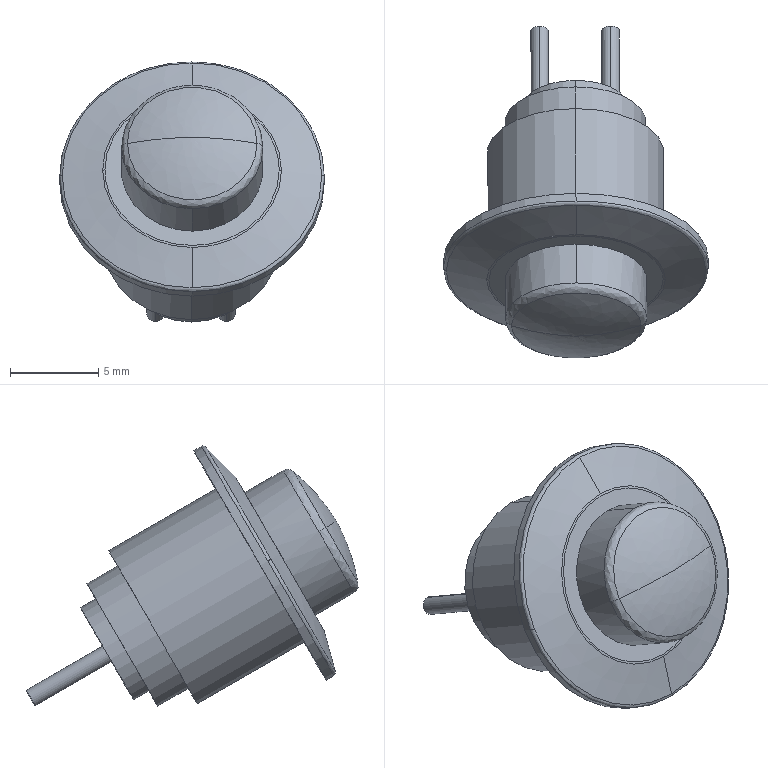Part | SolidWorks | features BaseBody 1 | 1 solid | 31 faces | box 15.002 x 18.816 x 14.734 mm | volume 1046 mm3 | cylinder 14 | spline 8 | plane 7 | cone 2 | commonest cylinder face diameters 1 x4 8 x4 6.02 x2 10 x2 15 x2
STEP:
#1=CARTESIAN_POINT('',(757.571,31.906,30.606));
#2=VERTEX_POINT('',#1);
#3=CARTESIAN_POINT('',(764.921,28.263,24.241));
#4=VERTEX_POINT('',#3);
#5=CARTESIAN_POINT('',(757.571,28.231,24.241));
#6=DIRECTION('',(-0.003769,0.866,-0.5));
#7=DIRECTION('',(-1.,-0.004352,0.000000001));
#8=AXIS2_PLACEMENT_3D('',#5,#6,#7);
#9=CIRCLE('',#8,7.35);
#10=EDGE_CURVE('',#2,#4,#9,.T.);
#11=ORIENTED_EDGE('',*,*,#10,.T.);
#12=CARTESIAN_POINT('',(765.07,28.431,24.144));
#13=VERTEX_POINT('',#12);
#14=CARTESIAN_POINT('',(764.87,28.43,24.144));
#15=DIRECTION('',(-0.002176,0.5,0.866));
#16=DIRECTION('',(1.,0.004352,-0.000000001));
#17=AXIS2_PLACEMENT_3D('',#14,#15,#16);
#18=CIRCLE('',#17,0.2);
#19=EDGE_CURVE('',#4,#13,#18,.T.);
#20=ORIENTED_EDGE('',*,*,#19,.T.);
#21=CARTESIAN_POINT('',(757.57,32.149,30.639));
#22=VERTEX_POINT('',#21);
#23=CARTESIAN_POINT('',(757.57,28.399,24.144));
#24=DIRECTION('',(-0.003769,0.866,-0.5));
#25=DIRECTION('',(0.,-0.5,-0.866));
#26=AXIS2_PLACEMENT_3D('',#23,#24,#25);
#27=CIRCLE('',#26,7.5);
#28=EDGE_CURVE('',#22,#13,#27,.T.);
#29=ORIENTED_EDGE('',*,*,#28,.F.);
#30=CARTESIAN_POINT('',(750.07,28.366,24.144));
#31=VERTEX_POINT('',#30);
#32=CARTESIAN_POINT('',(757.57,28.399,24.144));
#33=DIRECTION('',(-0.003769,0.866,-0.5));
#34=DIRECTION('',(0.,-0.5,-0.866));
#35=AXIS2_PLACEMENT_3D('',#32,#33,#34);
#36=CIRCLE('',#35,7.5);
#37=EDGE_CURVE('',#31,#22,#36,.T.);
#38=ORIENTED_EDGE('',*,*,#37,.F.);
#39=CARTESIAN_POINT('',(750.221,28.199,24.241));
#40=VERTEX_POINT('',#39);
#41=CARTESIAN_POINT('',(750.27,28.367,24.144));
#42=DIRECTION('',(0.002176,-0.5,-0.866));
#43=DIRECTION('',(-1.,-0.004352,0.000000001));
#44=AXIS2_PLACEMENT_3D('',#41,#42,#43);
#45=CIRCLE('',#44,0.2);
#46=EDGE_CURVE('',#40,#31,#45,.T.);
#47=ORIENTED_EDGE('',*,*,#46,.F.);
#48=CARTESIAN_POINT('',(757.571,28.231,24.241));
#49=DIRECTION('',(-0.003769,0.866,-0.5));
#50=DIRECTION('',(-1.,-0.004352,0.000000001));
#51=AXIS2_PLACEMENT_3D('',#48,#49,#50);
#52=CIRCLE('',#51,7.35);
#53=EDGE_CURVE('',#40,#2,#52,.T.);
#54=ORIENTED_EDGE('',*,*,#53,.T.);
#55=EDGE_LOOP('',(#11,#20,#29,#38,#47,#54));
#56=FACE_OUTER_BOUND('',#55,.T.);
#57=CARTESIAN_POINT('',(764.921,28.263,24.241));
#58=CARTESIAN_POINT('',(764.889,35.613,36.972));
#59=CARTESIAN_POINT('',(750.189,35.549,36.972));
#60=CARTESIAN_POINT('',(750.221,28.199,24.241));
#61=CARTESIAN_POINT('',(765.013,28.284,24.229));
#62=CARTESIAN_POINT('',(764.981,35.726,37.119));
#63=CARTESIAN_POINT('',(750.097,35.661,37.119));
#64=CARTESIAN_POINT('',(750.129,28.219,24.229));
#65=CARTESIAN_POINT('',(765.071,28.349,24.191));
#66=CARTESIAN_POINT('',(765.038,35.849,37.182));
#67=CARTESIAN_POINT('',(750.038,35.784,37.182));
#68=CARTESIAN_POINT('',(750.071,28.284,24.191));
#69=CARTESIAN_POINT('',(765.07,28.431,24.144));
#70=CARTESIAN_POINT('',(765.038,35.931,37.134));
#71=CARTESIAN_POINT('',(750.038,35.866,37.134));
#72=CARTESIAN_POINT('',(750.07,28.366,24.144));
#73=(BOUNDED_SURFACE()B_SPLINE_SURFACE(3,3,((#57,#58,#59,#60),(#61,#62,#63,#64),(#65,#66,#67,#68),(#69,#70,#71,#72)),.UNSPECIFIED.,.F.,.F.,.F.)B_SPLINE_SURFACE_WITH_KNOTS((4,4),(4,4),(0.,1.),(0.,1.),.UNSPECIFIED.)GEOMETRIC_REPRESENTATION_ITEM()RATIONAL_B_SPLINE_SURFACE(((1.,0.3333,0.3333,1.),(0.8607,0.2869,0.2869,0.8607),(0.8607,0.2869,0.2869,0.8607),(1.,0.3333,0.3333,1.)))REPRESENTATION_ITEM('')SURFACE());
#74=ADVANCED_FACE('',(#56),#73,.T.);
#75=CARTESIAN_POINT('',(752.637,27.68,24.546));
#76=VERTEX_POINT('',#75);
#77=CARTESIAN_POINT('',(762.509,27.723,24.546));
#78=VERTEX_POINT('',#77);
#79=CARTESIAN_POINT('',(752.637,27.68,24.546));
#80=CARTESIAN_POINT('',(752.616,32.616,33.096));
#81=CARTESIAN_POINT('',(762.488,32.659,33.096));
#82=CARTESIAN_POINT('',(762.509,27.723,24.546));
#83=(BOUNDED_CURVE()B_SPLINE_CURVE(3,(#79,#80,#81,#82),.UNSPECIFIED.,.F.,.F.)B_SPLINE_CURVE_WITH_KNOTS((4,4),(0.,1.),.UNSPECIFIED.)CURVE()GEOMETRIC_REPRESENTATION_ITEM()RATIONAL_B_SPLINE_CURVE((1.,0.3333,0.3333,1.))REPRESENTATION_ITEM(''));
#84=EDGE_CURVE('',#76,#78,#83,.T.);
#85=ORIENTED_EDGE('',*,*,#84,.T.);
#86=CARTESIAN_POINT('',(762.635,27.738,24.538));
#87=VERTEX_POINT('',#86);
#88=CARTESIAN_POINT('',(762.507,28.156,24.296));
#89=DIRECTION('',(-0.002176,0.5,0.866));
#90=DIRECTION('',(1.,0.004352,-0.000000001));
#91=AXIS2_PLACEMENT_3D('',#88,#89,#90);
#92=CIRCLE('',#91,0.5);
#93=EDGE_CURVE('',#78,#87,#92,.T.);
#94=ORIENTED_EDGE('',*,*,#93,.T.);
#95=CARTESIAN_POINT('',(757.573,30.247,28.922));
#96=VERTEX_POINT('',#95);
#97=CARTESIAN_POINT('',(757.573,27.716,24.538));
#98=DIRECTION('',(-0.003769,0.866,-0.5));
#99=DIRECTION('',(1.,0.004352,-0.000000001));
#100=AXIS2_PLACEMENT_3D('',#97,#98,#99);
#101=CIRCLE('',#100,5.062);
#102=EDGE_CURVE('',#96,#87,#101,.T.);
#103=ORIENTED_EDGE('',*,*,#102,.F.);
#104=CARTESIAN_POINT('',(752.511,27.694,24.538));
#105=VERTEX_POINT('',#104);
#106=CARTESIAN_POINT('',(757.573,27.716,24.538));
#107=DIRECTION('',(-0.003769,0.866,-0.5));
#108=DIRECTION('',(1.,0.004352,-0.000000001));
#109=AXIS2_PLACEMENT_3D('',#106,#107,#108);
#110=CIRCLE('',#109,5.062);
#111=EDGE_CURVE('',#105,#96,#110,.T.);
#112=ORIENTED_EDGE('',*,*,#111,.F.);
#113=CARTESIAN_POINT('',(752.635,28.113,24.296));
#114=DIRECTION('',(0.002176,-0.5,-0.866));
#115=DIRECTION('',(-1.,-0.004352,0.000000001));
#116=AXIS2_PLACEMENT_3D('',#113,#114,#115);
#117=CIRCLE('',#116,0.5);
#118=EDGE_CURVE('',#76,#105,#117,.T.);
#119=ORIENTED_EDGE('',*,*,#118,.F.);
#120=EDGE_LOOP('',(#85,#94,#103,#112,#119));
#121=FACE_OUTER_BOUND('',#120,.T.);
#122=CARTESIAN_POINT('',(762.509,27.723,24.546));
#123=CARTESIAN_POINT('',(762.488,32.659,33.096));
#124=CARTESIAN_POINT('',(752.616,32.616,33.096));
#125=CARTESIAN_POINT('',(752.637,27.68,24.546));
#126=CARTESIAN_POINT('',(762.552,27.723,24.546));
#127=CARTESIAN_POINT('',(762.53,32.702,33.169));
#128=CARTESIAN_POINT('',(752.573,32.659,33.169));
#129=CARTESIAN_POINT('',(752.595,27.68,24.546));
#130=CARTESIAN_POINT('',(762.594,27.728,24.543));
#131=CARTESIAN_POINT('',(762.572,32.749,33.24));
#132=CARTESIAN_POINT('',(752.531,32.705,33.24));
#133=CARTESIAN_POINT('',(752.553,27.684,24.543));
#134=CARTESIAN_POINT('',(762.635,27.738,24.538));
#135=CARTESIAN_POINT('',(762.613,32.799,33.305));
#136=CARTESIAN_POINT('',(752.489,32.755,33.305));
#137=CARTESIAN_POINT('',(752.511,27.694,24.538));
#138=(BOUNDED_SURFACE()B_SPLINE_SURFACE(3,3,((#122,#123,#124,#125),(#126,#127,#128,#129),(#130,#131,#132,#133),(#134,#135,#136,#137)),.UNSPECIFIED.,.F.,.F.,.F.)B_SPLINE_SURFACE_WITH_KNOTS((4,4),(4,4),(0.,1.),(0.,1.),.UNSPECIFIED.)GEOMETRIC_REPRESENTATION_ITEM()RATIONAL_B_SPLINE_SURFACE(((1.,0.3333,0.3333,1.),(0.9946,0.3315,0.3315,0.9946),(0.9946,0.3315,0.3315,0.9946),(1.,0.3333,0.3333,1.)))REPRESENTATION_ITEM('')SURFACE());
#139=ADVANCED_FACE('',(#121),#138,.T.);
#140=CARTESIAN_POINT('',(761.257,25.12,26.046));
#141=VERTEX_POINT('',#140);
#142=CARTESIAN_POINT('',(753.912,25.088,26.046));
#143=VERTEX_POINT('',#142);
#144=CARTESIAN_POINT('',(757.585,25.104,26.046));
#145=DIRECTION('',(-0.003769,0.866,-0.5));
#146=DIRECTION('',(1.,0.004352,-0.000000001));
#147=AXIS2_PLACEMENT_3D('',#144,#145,#146);
#148=CIRCLE('',#147,3.672);
#149=EDGE_CURVE('',#141,#143,#148,.T.);
#150=ORIENTED_EDGE('',*,*,#149,.T.);
#151=CARTESIAN_POINT('',(753.583,25.493,25.811));
#152=VERTEX_POINT('',#151);
#153=CARTESIAN_POINT('',(754.083,25.495,25.811));
#154=DIRECTION('',(0.002176,-0.5,-0.866));
#155=DIRECTION('',(-1.,-0.004352,0.000000001));
#156=AXIS2_PLACEMENT_3D('',#153,#154,#155);
#157=CIRCLE('',#156,0.5);
#158=EDGE_CURVE('',#143,#152,#157,.T.);
#159=ORIENTED_EDGE('',*,*,#158,.T.);
#160=CARTESIAN_POINT('',(757.583,23.51,22.347));
#161=VERTEX_POINT('',#160);
#162=CARTESIAN_POINT('',(757.583,25.51,25.811));
#163=DIRECTION('',(-0.003769,0.866,-0.5));
#164=DIRECTION('',(0.,-0.5,-0.866));
#165=AXIS2_PLACEMENT_3D('',#162,#163,#164);
#166=CIRCLE('',#165,4.);
#167=EDGE_CURVE('',#161,#152,#166,.T.);
#168=ORIENTED_EDGE('',*,*,#167,.F.);
#169=CARTESIAN_POINT('',(761.583,25.528,25.811));
#170=VERTEX_POINT('',#169);
#171=CARTESIAN_POINT('',(757.583,25.51,25.811));
#172=DIRECTION('',(-0.003769,0.866,-0.5));
#173=DIRECTION('',(0.,-0.5,-0.866));
#174=AXIS2_PLACEMENT_3D('',#171,#172,#173);
#175=CIRCLE('',#174,4.);
#176=EDGE_CURVE('',#170,#161,#175,.T.);
#177=ORIENTED_EDGE('',*,*,#176,.F.);
#178=CARTESIAN_POINT('',(761.083,25.525,25.811));
#179=DIRECTION('',(-0.002176,0.5,0.866));
#180=DIRECTION('',(1.,0.004352,-0.000000001));
#181=AXIS2_PLACEMENT_3D('',#178,#179,#180);
#182=CIRCLE('',#181,0.5);
#183=EDGE_CURVE('',#141,#170,#182,.T.);
#184=ORIENTED_EDGE('',*,*,#183,.F.);
#185=EDGE_LOOP('',(#150,#159,#168,#177,#184));
#186=FACE_OUTER_BOUND('',#185,.T.);
#187=CARTESIAN_POINT('',(753.912,25.088,26.046));
#188=CARTESIAN_POINT('',(753.928,21.415,19.685));
#189=CARTESIAN_POINT('',(761.273,21.447,19.685));
#190=CARTESIAN_POINT('',(761.257,25.12,26.046));
#191=CARTESIAN_POINT('',(753.709,25.152,26.009));
#192=CARTESIAN_POINT('',(753.725,21.276,19.295));
#193=CARTESIAN_POINT('',(761.477,21.31,19.295));
#194=CARTESIAN_POINT('',(761.46,25.185,26.009));
#195=CARTESIAN_POINT('',(753.584,25.305,25.92));
#196=CARTESIAN_POINT('',(753.601,21.305,18.992));
#197=CARTESIAN_POINT('',(761.601,21.34,18.992));
#198=CARTESIAN_POINT('',(761.584,25.34,25.92));
#199=CARTESIAN_POINT('',(753.583,25.493,25.811));
#200=CARTESIAN_POINT('',(753.6,21.493,18.883));
#201=CARTESIAN_POINT('',(761.6,21.528,18.883));
#202=CARTESIAN_POINT('',(761.583,25.528,25.811));
#203=(BOUNDED_SURFACE()B_SPLINE_SURFACE(3,3,((#187,#188,#189,#190),(#191,#192,#193,#194),(#195,#196,#197,#198),(#199,#200,#201,#202)),.UNSPECIFIED.,.F.,.F.,.T.)B_SPLINE_SURFACE_WITH_KNOTS((4,4),(4,4),(0.,1.),(0.,1.),.UNSPECIFIED.)GEOMETRIC_REPRESENTATION_ITEM()RATIONAL_B_SPLINE_SURFACE(((1.,0.3333,0.3333,1.),(0.88,0.2933,0.2933,0.88),(0.88,0.2933,0.2933,0.88),(1.,0.3333,0.3333,1.)))REPRESENTATION_ITEM('')SURFACE());
#204=ADVANCED_FACE('',(#186),#203,.T.);
#205=CARTESIAN_POINT('',(757.587,24.497,26.396));
#206=VERTEX_POINT('',#205);
#207=CARTESIAN_POINT('',(757.26,34.431,20.66));
#208=DIRECTION('',(-0.002176,0.5,0.866));
#209=DIRECTION('',(1.,0.004352,-0.000000001));
#210=AXIS2_PLACEMENT_3D('',#207,#208,#209);
#211=CIRCLE('',#210,11.475);
#212=EDGE_CURVE('',#206,#141,#211,.T.);
#213=ORIENTED_EDGE('',*,*,#212,.F.);
#214=CARTESIAN_POINT('',(757.828,34.433,20.66));
#215=DIRECTION('',(0.002176,-0.5,-0.866));
#216=DIRECTION('',(-1.,-0.004352,0.000000001));
#217=AXIS2_PLACEMENT_3D('',#214,#215,#216);
#218=CIRCLE('',#217,11.475);
#219=EDGE_CURVE('',#206,#143,#218,.T.);
#220=ORIENTED_EDGE('',*,*,#219,.T.);
#221=ORIENTED_EDGE('',*,*,#149,.F.);
#222=EDGE_LOOP('',(#213,#220,#221));
#223=FACE_OUTER_BOUND('',#222,.T.);
#224=CARTESIAN_POINT('',(757.587,24.497,26.396));
#225=CARTESIAN_POINT('',(757.587,24.497,26.396));
#226=CARTESIAN_POINT('',(757.587,24.497,26.396));
#227=CARTESIAN_POINT('',(757.587,24.497,26.396));
#228=CARTESIAN_POINT('',(756.33,24.519,26.38));
#229=CARTESIAN_POINT('',(756.336,23.262,24.203));
#230=CARTESIAN_POINT('',(758.85,23.273,24.203));
#231=CARTESIAN_POINT('',(758.844,24.53,26.38));
#232=CARTESIAN_POINT('',(755.094,24.717,26.263));
#233=CARTESIAN_POINT('',(755.105,22.225,21.946));
#234=CARTESIAN_POINT('',(760.089,22.247,21.946));
#235=CARTESIAN_POINT('',(760.078,24.739,26.263));
#236=CARTESIAN_POINT('',(753.912,25.088,26.046));
#237=CARTESIAN_POINT('',(753.928,21.415,19.685));
#238=CARTESIAN_POINT('',(761.273,21.447,19.685));
#239=CARTESIAN_POINT('',(761.257,25.12,26.046));
#240=(BOUNDED_SURFACE()B_SPLINE_SURFACE(3,3,((#224,#225,#226,#227),(#228,#229,#230,#231),(#232,#233,#234,#235),(#236,#237,#238,#239)),.UNSPECIFIED.,.F.,.F.,.T.)B_SPLINE_SURFACE_WITH_KNOTS((4,4),(4,4),(0.,1.),(0.,1.),.UNSPECIFIED.)GEOMETRIC_REPRESENTATION_ITEM()RATIONAL_B_SPLINE_SURFACE(((1.,0.3333,0.3333,1.),(0.9911,0.3304,0.3304,0.9911),(0.9911,0.3304,0.3304,0.9911),(1.,0.3333,0.3333,1.)))REPRESENTATION_ITEM('')SURFACE());
#241=ADVANCED_FACE('',(#223),#240,.T.);
#242=CARTESIAN_POINT('',(757.542,32.39,16.066));
#243=VERTEX_POINT('',#242);
#244=CARTESIAN_POINT('',(757.542,37.39,24.726));
#245=VERTEX_POINT('',#244);
#246=CARTESIAN_POINT('',(757.542,34.89,20.396));
#247=DIRECTION('',(0.003769,-0.866,0.5));
#248=DIRECTION('',(0.,-0.5,-0.866));
#249=AXIS2_PLACEMENT_3D('',#246,#247,#248);
#250=CIRCLE('',#249,5.);
#251=EDGE_CURVE('',#243,#245,#250,.T.);
#252=ORIENTED_EDGE('',*,*,#251,.T.);
#253=CARTESIAN_POINT('',(757.568,31.328,28.226));
#254=VERTEX_POINT('',#253);
#255=CARTESIAN_POINT('',(757.555,34.359,26.476));
#256=DIRECTION('',(0.003769,-0.866,0.5));
#257=VECTOR('',#256,1000.);
#258=LINE('',#255,#257);
#259=EDGE_CURVE('',#245,#254,#258,.T.);
#260=ORIENTED_EDGE('',*,*,#259,.T.);
#261=CARTESIAN_POINT('',(757.568,26.327,19.566));
#262=VERTEX_POINT('',#261);
#263=CARTESIAN_POINT('',(757.568,28.827,23.896));
#264=DIRECTION('',(-0.003769,0.866,-0.5));
#265=DIRECTION('',(0.,-0.5,-0.866));
#266=AXIS2_PLACEMENT_3D('',#263,#264,#265);
#267=CIRCLE('',#266,5.);
#268=EDGE_CURVE('',#254,#262,#267,.T.);
#269=ORIENTED_EDGE('',*,*,#268,.T.);
#270=CARTESIAN_POINT('',(757.555,29.359,17.816));
#271=DIRECTION('',(0.003769,-0.866,0.5));
#272=VECTOR('',#271,1000.);
#273=LINE('',#270,#272);
#274=EDGE_CURVE('',#243,#262,#273,.T.);
#275=ORIENTED_EDGE('',*,*,#274,.F.);
#276=EDGE_LOOP('',(#252,#260,#269,#275));
#277=FACE_OUTER_BOUND('',#276,.T.);
#278=CARTESIAN_POINT('',(757.555,31.859,22.146));
#279=DIRECTION('',(0.003769,-0.866,0.5));
#280=DIRECTION('',(0.,-0.5,-0.866));
#281=AXIS2_PLACEMENT_3D('',#278,#279,#280);
#282=CYLINDRICAL_SURFACE('',#281,5.);
#283=ADVANCED_FACE('',(#277),#282,.T.);
#284=CARTESIAN_POINT('',(757.568,32.578,30.391));
#285=VERTEX_POINT('',#284);
#286=CARTESIAN_POINT('',(757.568,25.077,17.401));
#287=VERTEX_POINT('',#286);
#288=CARTESIAN_POINT('',(757.568,28.827,23.896));
#289=DIRECTION('',(-0.003769,0.866,-0.5));
#290=DIRECTION('',(0.,-0.5,-0.866));
#291=AXIS2_PLACEMENT_3D('',#288,#289,#290);
#292=CIRCLE('',#291,7.5);
#293=EDGE_CURVE('',#285,#287,#292,.T.);
#294=ORIENTED_EDGE('',*,*,#293,.F.);
#295=CARTESIAN_POINT('',(757.57,32.296,30.554));
#296=DIRECTION('',(0.003769,-0.866,0.5));
#297=VECTOR('',#296,1000.);
#298=LINE('',#295,#297);
#299=EDGE_CURVE('',#285,#22,#298,.T.);
#300=ORIENTED_EDGE('',*,*,#299,.T.);
#301=ORIENTED_EDGE('',*,*,#28,.T.);
#302=CARTESIAN_POINT('',(757.57,24.648,17.649));
#303=VERTEX_POINT('',#302);
#304=CARTESIAN_POINT('',(757.57,28.399,24.144));
#305=DIRECTION('',(-0.003769,0.866,-0.5));
#306=DIRECTION('',(0.,-0.5,-0.866));
#307=AXIS2_PLACEMENT_3D('',#304,#305,#306);
#308=CIRCLE('',#307,7.5);
#309=EDGE_CURVE('',#13,#303,#308,.T.);
#310=ORIENTED_EDGE('',*,*,#309,.T.);
#311=CARTESIAN_POINT('',(757.57,24.796,17.563));
#312=DIRECTION('',(0.003769,-0.866,0.5));
#313=VECTOR('',#312,1000.);
#314=LINE('',#311,#313);
#315=EDGE_CURVE('',#287,#303,#314,.T.);
#316=ORIENTED_EDGE('',*,*,#315,.F.);
#317=EDGE_LOOP('',(#294,#300,#301,#310,#316));
#318=FACE_OUTER_BOUND('',#317,.T.);
#319=CARTESIAN_POINT('',(757.57,28.546,24.059));
#320=DIRECTION('',(0.003769,-0.866,0.5));
#321=DIRECTION('',(0.,-0.5,-0.866));
#322=AXIS2_PLACEMENT_3D('',#319,#320,#321);
#323=CYLINDRICAL_SURFACE('',#322,7.5);
#324=ADVANCED_FACE('',(#318),#323,.T.);
#325=CARTESIAN_POINT('',(757.535,34.622,15.932));
#326=VERTEX_POINT('',#325);
#327=CARTESIAN_POINT('',(757.535,38.622,22.86));
#328=VERTEX_POINT('',#327);
#329=CARTESIAN_POINT('',(757.535,36.622,19.396));
#330=DIRECTION('',(0.003769,-0.866,0.5));
#331=DIRECTION('',(0.,-0.5,-0.866));
#332=AXIS2_PLACEMENT_3D('',#329,#330,#331);
#333=CIRCLE('',#332,4.);
#334=EDGE_CURVE('',#326,#328,#333,.T.);
#335=ORIENTED_EDGE('',*,*,#334,.T.);
#336=CARTESIAN_POINT('',(757.542,36.89,23.86));
#337=VERTEX_POINT('',#336);
#338=CARTESIAN_POINT('',(757.538,37.756,23.36));
#339=DIRECTION('',(0.003769,-0.866,0.5));
#340=VECTOR('',#339,1000.);
#341=LINE('',#338,#340);
#342=EDGE_CURVE('',#328,#337,#341,.T.);
#343=ORIENTED_EDGE('',*,*,#342,.T.);
#344=CARTESIAN_POINT('',(757.542,32.89,16.932));
#345=VERTEX_POINT('',#344);
#346=CARTESIAN_POINT('',(757.542,34.89,20.396));
#347=DIRECTION('',(0.003769,-0.866,0.5));
#348=DIRECTION('',(0.,-0.5,-0.866));
#349=AXIS2_PLACEMENT_3D('',#346,#347,#348);
#350=CIRCLE('',#349,4.);
#351=EDGE_CURVE('',#345,#337,#350,.T.);
#352=ORIENTED_EDGE('',*,*,#351,.F.);
#353=CARTESIAN_POINT('',(757.538,33.756,16.432));
#354=DIRECTION('',(0.003769,-0.866,0.5));
#355=VECTOR('',#354,1000.);
#356=LINE('',#353,#355);
#357=EDGE_CURVE('',#326,#345,#356,.T.);
#358=ORIENTED_EDGE('',*,*,#357,.F.);
#359=EDGE_LOOP('',(#335,#343,#352,#358));
#360=FACE_OUTER_BOUND('',#359,.T.);
#361=CARTESIAN_POINT('',(757.538,35.756,19.896));
#362=DIRECTION('',(0.003769,-0.866,0.5));
#363=DIRECTION('',(0.,-0.5,-0.866));
#364=AXIS2_PLACEMENT_3D('',#361,#362,#363);
#365=CYLINDRICAL_SURFACE('',#364,4.);
#366=ADVANCED_FACE('',(#360),#365,.T.);
#367=ORIENTED_EDGE('',*,*,#102,.T.);
#368=CARTESIAN_POINT('',(757.573,25.185,20.154));
#369=VERTEX_POINT('',#368);
#370=CARTESIAN_POINT('',(757.573,27.716,24.538));
#371=DIRECTION('',(-0.003769,0.866,-0.5));
#372=DIRECTION('',(1.,0.004352,-0.000000001));
#373=AXIS2_PLACEMENT_3D('',#370,#371,#372);
#374=CIRCLE('',#373,5.062);
#375=EDGE_CURVE('',#87,#369,#374,.T.);
#376=ORIENTED_EDGE('',*,*,#375,.T.);
#377=CARTESIAN_POINT('',(757.571,24.556,17.875));
#378=VERTEX_POINT('',#377);
#379=CARTESIAN_POINT('',(757.571,24.556,17.875));
#380=DIRECTION('',(-0.0009484,-0.266,-0.964));
#381=VECTOR('',#380,1000.);
#382=LINE('',#379,#381);
#383=EDGE_CURVE('',#369,#378,#382,.T.);
#384=ORIENTED_EDGE('',*,*,#383,.T.);
#385=CARTESIAN_POINT('',(757.571,28.231,24.241));
#386=DIRECTION('',(-0.003769,0.866,-0.5));
#387=DIRECTION('',(-1.,-0.004352,0.000000001));
#388=AXIS2_PLACEMENT_3D('',#385,#386,#387);
#389=CIRCLE('',#388,7.35);
#390=EDGE_CURVE('',#4,#378,#389,.T.);
#391=ORIENTED_EDGE('',*,*,#390,.F.);
#392=ORIENTED_EDGE('',*,*,#10,.F.);
#393=CARTESIAN_POINT('',(757.571,31.906,30.606));
#394=DIRECTION('',(-0.0009484,0.7018,0.7123));
#395=VECTOR('',#394,1000.);
#396=LINE('',#393,#395);
#397=EDGE_CURVE('',#96,#2,#396,.T.);
#398=ORIENTED_EDGE('',*,*,#397,.F.);
#399=EDGE_LOOP('',(#367,#376,#384,#391,#392,#398));
#400=FACE_OUTER_BOUND('',#399,.T.);
#401=CARTESIAN_POINT('',(757.571,28.231,24.241));
#402=DIRECTION('',(-0.003769,0.866,-0.5));
#403=DIRECTION('',(0.,0.5,0.866));
#404=AXIS2_PLACEMENT_3D('',#401,#402,#403);
#405=CONICAL_SURFACE('',#404,7.35,1.316);
#406=ADVANCED_FACE('',(#400),#405,.T.);
#407=CARTESIAN_POINT('',(757.531,35.983,16.289));
#408=VERTEX_POINT('',#407);
#409=CARTESIAN_POINT('',(757.531,38.993,21.503));
#410=VERTEX_POINT('',#409);
#411=CARTESIAN_POINT('',(757.531,37.488,18.896));
#412=DIRECTION('',(0.003769,-0.866,0.5));
#413=DIRECTION('',(0.,-0.5,-0.866));
#414=AXIS2_PLACEMENT_3D('',#411,#412,#413);
#415=CIRCLE('',#414,3.01);
#416=EDGE_CURVE('',#408,#410,#415,.T.);
#417=ORIENTED_EDGE('',*,*,#416,.T.);
#418=CARTESIAN_POINT('',(757.535,38.127,22.003));
#419=VERTEX_POINT('',#418);
#420=CARTESIAN_POINT('',(757.533,38.56,21.753));
#421=DIRECTION('',(0.003769,-0.866,0.5));
#422=VECTOR('',#421,1000.);
#423=LINE('',#420,#422);
#424=EDGE_CURVE('',#410,#419,#423,.T.);
#425=ORIENTED_EDGE('',*,*,#424,.T.);
#426=CARTESIAN_POINT('',(757.535,35.117,16.789));
#427=VERTEX_POINT('',#426);
#428=CARTESIAN_POINT('',(757.535,36.622,19.396));
#429=DIRECTION('',(0.003769,-0.866,0.5));
#430=DIRECTION('',(0.,-0.5,-0.866));
#431=AXIS2_PLACEMENT_3D('',#428,#429,#430);
#432=CIRCLE('',#431,3.01);
#433=EDGE_CURVE('',#427,#419,#432,.T.);
#434=ORIENTED_EDGE('',*,*,#433,.F.);
#435=CARTESIAN_POINT('',(757.533,35.55,16.539));
#436=DIRECTION('',(0.003769,-0.866,0.5));
#437=VECTOR('',#436,1000.);
#438=LINE('',#435,#437);
#439=EDGE_CURVE('',#408,#427,#438,.T.);
#440=ORIENTED_EDGE('',*,*,#439,.F.);
#441=EDGE_LOOP('',(#417,#425,#434,#440));
#442=FACE_OUTER_BOUND('',#441,.T.);
#443=CARTESIAN_POINT('',(757.533,37.055,19.146));
#444=DIRECTION('',(0.003769,-0.866,0.5));
#445=DIRECTION('',(0.,-0.5,-0.866));
#446=AXIS2_PLACEMENT_3D('',#443,#444,#445);
#447=CYLINDRICAL_SURFACE('',#446,3.01);
#448=ADVANCED_FACE('',(#442),#447,.T.);
#449=CARTESIAN_POINT('',(759.512,41.576,15.963));
#450=VERTEX_POINT('',#449);
#451=CARTESIAN_POINT('',(759.512,42.076,16.829));
#452=VERTEX_POINT('',#451);
#453=CARTESIAN_POINT('',(759.512,41.826,16.396));
#454=DIRECTION('',(0.003769,-0.866,0.5));
#455=DIRECTION('',(0.,-0.5,-0.866));
#456=AXIS2_PLACEMENT_3D('',#453,#454,#455);
#457=CIRCLE('',#456,0.5);
#458=EDGE_CURVE('',#450,#452,#457,.T.);
#459=ORIENTED_EDGE('',*,*,#458,.T.);
#460=CARTESIAN_POINT('',(759.531,37.746,19.329));
#461=VERTEX_POINT('',#460);
#462=CARTESIAN_POINT('',(759.531,37.746,19.329));
#463=DIRECTION('',(0.003769,-0.866,0.5));
#464=VECTOR('',#463,1000.);
#465=LINE('',#462,#464);
#466=EDGE_CURVE('',#452,#461,#465,.T.);
#467=ORIENTED_EDGE('',*,*,#466,.T.);
#468=CARTESIAN_POINT('',(759.531,37.246,18.463));
#469=VERTEX_POINT('',#468);
#470=CARTESIAN_POINT('',(759.531,37.496,18.896));
#471=DIRECTION('',(0.003769,-0.866,0.5));
#472=DIRECTION('',(0.,-0.5,-0.866));
#473=AXIS2_PLACEMENT_3D('',#470,#471,#472);
#474=CIRCLE('',#473,0.5);
#475=EDGE_CURVE('',#469,#461,#474,.T.);
#476=ORIENTED_EDGE('',*,*,#475,.F.);
#477=CARTESIAN_POINT('',(759.531,37.246,18.463));
#478=DIRECTION('',(0.003769,-0.866,0.5));
#479=VECTOR('',#478,1000.);
#480=LINE('',#477,#479);
#481=EDGE_CURVE('',#450,#469,#480,.T.);
#482=ORIENTED_EDGE('',*,*,#481,.F.);
#483=EDGE_LOOP('',(#459,#467,#476,#482));
#484=FACE_OUTER_BOUND('',#483,.T.);
#485=CARTESIAN_POINT('',(759.531,37.496,18.896));
#486=DIRECTION('',(0.003769,-0.866,0.5));
#487=DIRECTION('',(0.,-0.5,-0.866));
#488=AXIS2_PLACEMENT_3D('',#485,#486,#487);
#489=CYLINDRICAL_SURFACE('',#488,0.5);
#490=ADVANCED_FACE('',(#484),#489,.T.);
#491=CARTESIAN_POINT('',(755.512,41.559,15.963));
#492=VERTEX_POINT('',#491);
#493=CARTESIAN_POINT('',(755.512,42.059,16.829));
#494=VERTEX_POINT('',#493);
#495=CARTESIAN_POINT('',(755.512,41.809,16.396));
#496=DIRECTION('',(0.003769,-0.866,0.5));
#497=DIRECTION('',(0.,-0.5,-0.866));
#498=AXIS2_PLACEMENT_3D('',#495,#496,#497);
#499=CIRCLE('',#498,0.5);
#500=EDGE_CURVE('',#492,#494,#499,.T.);
#501=ORIENTED_EDGE('',*,*,#500,.T.);
#502=CARTESIAN_POINT('',(755.531,37.729,19.329));
#503=VERTEX_POINT('',#502);
#504=CARTESIAN_POINT('',(755.531,37.729,19.329));
#505=DIRECTION('',(0.003769,-0.866,0.5));
#506=VECTOR('',#505,1000.);
#507=LINE('',#504,#506);
#508=EDGE_CURVE('',#494,#503,#507,.T.);
#509=ORIENTED_EDGE('',*,*,#508,.T.);
#510=CARTESIAN_POINT('',(755.531,37.229,18.463));
#511=VERTEX_POINT('',#510);
#512=CARTESIAN_POINT('',(755.531,37.479,18.896));
#513=DIRECTION('',(0.003769,-0.866,0.5));
#514=DIRECTION('',(0.,-0.5,-0.866));
#515=AXIS2_PLACEMENT_3D('',#512,#513,#514);
#516=CIRCLE('',#515,0.5);
#517=EDGE_CURVE('',#511,#503,#516,.T.);
#518=ORIENTED_EDGE('',*,*,#517,.F.);
#519=CARTESIAN_POINT('',(755.531,37.229,18.463));
#520=DIRECTION('',(0.003769,-0.866,0.5));
#521=VECTOR('',#520,1000.);
#522=LINE('',#519,#521);
#523=EDGE_CURVE('',#492,#511,#522,.T.);
#524=ORIENTED_EDGE('',*,*,#523,.F.);
#525=EDGE_LOOP('',(#501,#509,#518,#524));
#526=FACE_OUTER_BOUND('',#525,.T.);
#527=CARTESIAN_POINT('',(755.531,37.479,18.896));
#528=DIRECTION('',(0.003769,-0.866,0.5));
#529=DIRECTION('',(0.,-0.5,-0.866));
#530=AXIS2_PLACEMENT_3D('',#527,#528,#529);
#531=CYLINDRICAL_SURFACE('',#530,0.5);
#532=ADVANCED_FACE('',(#526),#531,.T.);
#533=CARTESIAN_POINT('',(757.573,29.702,28.01));
#534=VERTEX_POINT('',#533);
#535=CARTESIAN_POINT('',(757.573,25.702,21.082));
#536=VERTEX_POINT('',#535);
#537=CARTESIAN_POINT('',(757.573,27.702,24.546));
#538=DIRECTION('',(-0.003769,0.866,-0.5));
#539=DIRECTION('',(0.,-0.5,-0.866));
#540=AXIS2_PLACEMENT_3D('',#537,#538,#539);
#541=CIRCLE('',#540,4.);
#542=EDGE_CURVE('',#534,#536,#541,.T.);
#543=ORIENTED_EDGE('',*,*,#542,.F.);
#544=CARTESIAN_POINT('',(757.583,27.51,29.275));
#545=VERTEX_POINT('',#544);
#546=CARTESIAN_POINT('',(757.579,28.457,28.729));
#547=DIRECTION('',(0.003769,-0.866,0.5));
#548=VECTOR('',#547,1000.);
#549=LINE('',#546,#548);
#550=EDGE_CURVE('',#534,#545,#549,.T.);
#551=ORIENTED_EDGE('',*,*,#550,.T.);
#552=CARTESIAN_POINT('',(757.583,25.51,25.811));
#553=DIRECTION('',(-0.003769,0.866,-0.5));
#554=DIRECTION('',(0.,-0.5,-0.866));
#555=AXIS2_PLACEMENT_3D('',#552,#553,#554);
#556=CIRCLE('',#555,4.);
#557=EDGE_CURVE('',#545,#170,#556,.T.);
#558=ORIENTED_EDGE('',*,*,#557,.T.);
#559=ORIENTED_EDGE('',*,*,#176,.T.);
#560=CARTESIAN_POINT('',(757.579,24.457,21.8));
#561=DIRECTION('',(0.003769,-0.866,0.5));
#562=VECTOR('',#561,1000.);
#563=LINE('',#560,#562);
#564=EDGE_CURVE('',#536,#161,#563,.T.);
#565=ORIENTED_EDGE('',*,*,#564,.F.);
#566=EDGE_LOOP('',(#543,#551,#558,#559,#565));
#567=FACE_OUTER_BOUND('',#566,.T.);
#568=CARTESIAN_POINT('',(757.579,26.457,25.265));
#569=DIRECTION('',(0.003769,-0.866,0.5));
#570=DIRECTION('',(0.,-0.5,-0.866));
#571=AXIS2_PLACEMENT_3D('',#568,#569,#570);
#572=CYLINDRICAL_SURFACE('',#571,4.);
#573=ADVANCED_FACE('',(#567),#572,.T.);
#574=ORIENTED_EDGE('',*,*,#259,.F.);
#575=CARTESIAN_POINT('',(757.542,34.89,20.396));
#576=DIRECTION('',(0.003769,-0.866,0.5));
#577=DIRECTION('',(0.,-0.5,-0.866));
#578=AXIS2_PLACEMENT_3D('',#575,#576,#577);
#579=CIRCLE('',#578,5.);
#580=EDGE_CURVE('',#245,#243,#579,.T.);
#581=ORIENTED_EDGE('',*,*,#580,.T.);
#582=ORIENTED_EDGE('',*,*,#274,.T.);
#583=CARTESIAN_POINT('',(757.568,28.827,23.896));
#584=DIRECTION('',(-0.003769,0.866,-0.5));
#585=DIRECTION('',(0.,-0.5,-0.866));
#586=AXIS2_PLACEMENT_3D('',#583,#584,#585);
#587=CIRCLE('',#586,5.);
#588=EDGE_CURVE('',#262,#254,#587,.T.);
#589=ORIENTED_EDGE('',*,*,#588,.T.);
#590=EDGE_LOOP('',(#574,#581,#582,#589));
#591=FACE_OUTER_BOUND('',#590,.T.);
#592=CARTESIAN_POINT('',(757.555,31.859,22.146));
#593=DIRECTION('',(0.003769,-0.866,0.5));
#594=DIRECTION('',(0.,-0.5,-0.866));
#595=AXIS2_PLACEMENT_3D('',#592,#593,#594);
#596=CYLINDRICAL_SURFACE('',#595,5.);
#597=ADVANCED_FACE('',(#591),#596,.T.);
#598=CARTESIAN_POINT('',(757.568,28.827,23.896));
#599=DIRECTION('',(-0.003769,0.866,-0.5));
#600=DIRECTION('',(0.,-0.5,-0.866));
#601=AXIS2_PLACEMENT_3D('',#598,#599,#600);
#602=CIRCLE('',#601,7.5);
#603=EDGE_CURVE('',#287,#285,#602,.T.);
#604=ORIENTED_EDGE('',*,*,#603,.T.);
#605=ORIENTED_EDGE('',*,*,#293,.T.);
#606=EDGE_LOOP('',(#604,#605));
#607=FACE_OUTER_BOUND('',#606,.T.);
#608=ORIENTED_EDGE('',*,*,#588,.F.);
#609=ORIENTED_EDGE('',*,*,#268,.F.);
#610=EDGE_LOOP('',(#608,#609));
#611=FACE_BOUND('',#610,.T.);
#612=CARTESIAN_POINT('',(763.818,28.855,23.896));
#613=DIRECTION('',(-0.003769,0.866,-0.5));
#614=DIRECTION('',(0.,0.5,0.866));
#615=AXIS2_PLACEMENT_3D('',#612,#613,#614);
#616=PLANE('',#615);
#617=ADVANCED_FACE('',(#607,#611),#616,.T.);
#618=ORIENTED_EDGE('',*,*,#251,.F.);
#619=ORIENTED_EDGE('',*,*,#580,.F.);
#620=EDGE_LOOP('',(#618,#619));
#621=FACE_OUTER_BOUND('',#620,.T.);
#622=ORIENTED_EDGE('',*,*,#351,.T.);
#623=CARTESIAN_POINT('',(757.542,34.89,20.396));
#624=DIRECTION('',(0.003769,-0.866,0.5));
#625=DIRECTION('',(0.,-0.5,-0.866));
#626=AXIS2_PLACEMENT_3D('',#623,#624,#625);
#627=CIRCLE('',#626,4.);
#628=EDGE_CURVE('',#337,#345,#627,.T.);
#629=ORIENTED_EDGE('',*,*,#628,.T.);
#630=EDGE_LOOP('',(#622,#629));
#631=FACE_BOUND('',#630,.T.);
#632=CARTESIAN_POINT('',(762.042,34.909,20.396));
#633=DIRECTION('',(-0.003769,0.866,-0.5));
#634=DIRECTION('',(0.,0.5,0.866));
#635=AXIS2_PLACEMENT_3D('',#632,#633,#634);
#636=PLANE('',#635);
#637=ADVANCED_FACE('',(#621,#631),#636,.T.);
#638=ORIENTED_EDGE('',*,*,#299,.F.);
#639=ORIENTED_EDGE('',*,*,#603,.F.);
#640=ORIENTED_EDGE('',*,*,#315,.T.);
#641=CARTESIAN_POINT('',(757.57,28.399,24.144));
#642=DIRECTION('',(-0.003769,0.866,-0.5));
#643=DIRECTION('',(0.,-0.5,-0.866));
#644=AXIS2_PLACEMENT_3D('',#641,#642,#643);
#645=CIRCLE('',#644,7.5);
#646=EDGE_CURVE('',#303,#31,#645,.T.);
#647=ORIENTED_EDGE('',*,*,#646,.T.);
#648=ORIENTED_EDGE('',*,*,#37,.T.);
#649=EDGE_LOOP('',(#638,#639,#640,#647,#648));
#650=FACE_OUTER_BOUND('',#649,.T.);
#651=CARTESIAN_POINT('',(757.57,28.546,24.059));
#652=DIRECTION('',(0.003769,-0.866,0.5));
#653=DIRECTION('',(0.,-0.5,-0.866));
#654=AXIS2_PLACEMENT_3D('',#651,#652,#653);
#655=CYLINDRICAL_SURFACE('',#654,7.5);
#656=ADVANCED_FACE('',(#650),#655,.T.);
#657=ORIENTED_EDGE('',*,*,#342,.F.);
#658=CARTESIAN_POINT('',(757.535,36.622,19.396));
#659=DIRECTION('',(0.003769,-0.866,0.5));
#660=DIRECTION('',(0.,-0.5,-0.866));
#661=AXIS2_PLACEMENT_3D('',#658,#659,#660);
#662=CIRCLE('',#661,4.);
#663=EDGE_CURVE('',#328,#326,#662,.T.);
#664=ORIENTED_EDGE('',*,*,#663,.T.);
#665=ORIENTED_EDGE('',*,*,#357,.T.);
#666=ORIENTED_EDGE('',*,*,#628,.F.);
#667=EDGE_LOOP('',(#657,#664,#665,#666));
#668=FACE_OUTER_BOUND('',#667,.T.);
#669=CARTESIAN_POINT('',(757.538,35.756,19.896));
#670=DIRECTION('',(0.003769,-0.866,0.5));
#671=DIRECTION('',(0.,-0.5,-0.866));
#672=AXIS2_PLACEMENT_3D('',#669,#670,#671);
#673=CYLINDRICAL_SURFACE('',#672,4.);
#674=ADVANCED_FACE('',(#668),#673,.T.);
#675=ORIENTED_EDGE('',*,*,#19,.F.);
#676=ORIENTED_EDGE('',*,*,#390,.T.);
#677=CARTESIAN_POINT('',(757.571,28.231,24.241));
#678=DIRECTION('',(-0.003769,0.866,-0.5));
#679=DIRECTION('',(-1.,-0.004352,0.000000001));
#680=AXIS2_PLACEMENT_3D('',#677,#678,#679);
#681=CIRCLE('',#680,7.35);
#682=EDGE_CURVE('',#378,#40,#681,.T.);
#683=ORIENTED_EDGE('',*,*,#682,.T.);
#684=ORIENTED_EDGE('',*,*,#46,.T.);
#685=ORIENTED_EDGE('',*,*,#646,.F.);
#686=ORIENTED_EDGE('',*,*,#309,.F.);
#687=EDGE_LOOP('',(#675,#676,#683,#684,#685,#686));
#688=FACE_OUTER_BOUND('',#687,.T.);
#689=CARTESIAN_POINT('',(750.221,28.199,24.241));
#690=CARTESIAN_POINT('',(750.253,20.849,11.509));
#691=CARTESIAN_POINT('',(764.953,20.913,11.509));
#692=CARTESIAN_POINT('',(764.921,28.263,24.241));
#693=CARTESIAN_POINT('',(750.129,28.219,24.229));
#694=CARTESIAN_POINT('',(750.161,20.777,11.339));
#695=CARTESIAN_POINT('',(765.045,20.842,11.339));
#696=CARTESIAN_POINT('',(765.013,28.284,24.229));
#697=CARTESIAN_POINT('',(750.071,28.284,24.191));
#698=CARTESIAN_POINT('',(750.103,20.784,11.201));
#699=CARTESIAN_POINT('',(765.103,20.849,11.201));
#700=CARTESIAN_POINT('',(765.071,28.349,24.191));
#701=CARTESIAN_POINT('',(750.07,28.366,24.144));
#702=CARTESIAN_POINT('',(750.103,20.866,11.153));
#703=CARTESIAN_POINT('',(765.103,20.931,11.153));
#704=CARTESIAN_POINT('',(765.07,28.431,24.144));
#705=(BOUNDED_SURFACE()B_SPLINE_SURFACE(3,3,((#689,#690,#691,#692),(#693,#694,#695,#696),(#697,#698,#699,#700),(#701,#702,#703,#704)),.UNSPECIFIED.,.F.,.F.,.F.)B_SPLINE_SURFACE_WITH_KNOTS((4,4),(4,4),(0.,1.),(0.,1.),.UNSPECIFIED.)GEOMETRIC_REPRESENTATION_ITEM()RATIONAL_B_SPLINE_SURFACE(((1.,0.3333,0.3333,1.),(0.8607,0.2869,0.2869,0.8607),(0.8607,0.2869,0.2869,0.8607),(1.,0.3333,0.3333,1.)))REPRESENTATION_ITEM('')SURFACE());
#706=ADVANCED_FACE('',(#688),#705,.T.);
#707=ORIENTED_EDGE('',*,*,#334,.F.);
#708=ORIENTED_EDGE('',*,*,#663,.F.);
#709=EDGE_LOOP('',(#707,#708));
#710=FACE_OUTER_BOUND('',#709,.T.);
#711=ORIENTED_EDGE('',*,*,#433,.T.);
#712=CARTESIAN_POINT('',(757.535,36.622,19.396));
#713=DIRECTION('',(0.003769,-0.866,0.5));
#714=DIRECTION('',(0.,-0.5,-0.866));
#715=AXIS2_PLACEMENT_3D('',#712,#713,#714);
#716=CIRCLE('',#715,3.01);
#717=EDGE_CURVE('',#419,#427,#716,.T.);
#718=ORIENTED_EDGE('',*,*,#717,.T.);
#719=EDGE_LOOP('',(#711,#718));
#720=FACE_BOUND('',#719,.T.);
#721=CARTESIAN_POINT('',(761.039,36.637,19.396));
#722=DIRECTION('',(-0.003769,0.866,-0.5));
#723=DIRECTION('',(0.,0.5,0.866));
#724=AXIS2_PLACEMENT_3D('',#721,#722,#723);
#725=PLANE('',#724);
#726=ADVANCED_FACE('',(#710,#720),#725,.T.);
#727=ORIENTED_EDGE('',*,*,#383,.F.);
#728=CARTESIAN_POINT('',(757.573,27.716,24.538));
#729=DIRECTION('',(-0.003769,0.866,-0.5));
#730=DIRECTION('',(1.,0.004352,-0.000000001));
#731=AXIS2_PLACEMENT_3D('',#728,#729,#730);
#732=CIRCLE('',#731,5.062);
#733=EDGE_CURVE('',#369,#105,#732,.T.);
#734=ORIENTED_EDGE('',*,*,#733,.T.);
#735=ORIENTED_EDGE('',*,*,#111,.T.);
#736=ORIENTED_EDGE('',*,*,#397,.T.);
#737=ORIENTED_EDGE('',*,*,#53,.F.);
#738=ORIENTED_EDGE('',*,*,#682,.F.);
#739=EDGE_LOOP('',(#727,#734,#735,#736,#737,#738));
#740=FACE_OUTER_BOUND('',#739,.T.);
#741=CARTESIAN_POINT('',(757.571,28.231,24.241));
#742=DIRECTION('',(-0.003769,0.866,-0.5));
#743=DIRECTION('',(0.,0.5,0.866));
#744=AXIS2_PLACEMENT_3D('',#741,#742,#743);
#745=CONICAL_SURFACE('',#744,7.35,1.316);
#746=ADVANCED_FACE('',(#740),#745,.T.);
#747=ORIENTED_EDGE('',*,*,#424,.F.);
#748=CARTESIAN_POINT('',(757.531,37.488,18.896));
#749=DIRECTION('',(0.003769,-0.866,0.5));
#750=DIRECTION('',(0.,-0.5,-0.866));
#751=AXIS2_PLACEMENT_3D('',#748,#749,#750);
#752=CIRCLE('',#751,3.01);
#753=EDGE_CURVE('',#410,#408,#752,.T.);
#754=ORIENTED_EDGE('',*,*,#753,.T.);
#755=ORIENTED_EDGE('',*,*,#439,.T.);
#756=ORIENTED_EDGE('',*,*,#717,.F.);
#757=EDGE_LOOP('',(#747,#754,#755,#756));
#758=FACE_OUTER_BOUND('',#757,.T.);
#759=CARTESIAN_POINT('',(757.533,37.055,19.146));
#760=DIRECTION('',(0.003769,-0.866,0.5));
#761=DIRECTION('',(0.,-0.5,-0.866));
#762=AXIS2_PLACEMENT_3D('',#759,#760,#761);
#763=CYLINDRICAL_SURFACE('',#762,3.01);
#764=ADVANCED_FACE('',(#758),#763,.T.);
#765=ORIENTED_EDGE('',*,*,#93,.F.);
#766=CARTESIAN_POINT('',(762.509,27.723,24.546));
#767=CARTESIAN_POINT('',(762.531,22.787,15.997));
#768=CARTESIAN_POINT('',(752.659,22.744,15.997));
#769=CARTESIAN_POINT('',(752.637,27.68,24.546));
#770=(BOUNDED_CURVE()B_SPLINE_CURVE(3,(#766,#767,#768,#769),.UNSPECIFIED.,.F.,.T.)B_SPLINE_CURVE_WITH_KNOTS((4,4),(0.,1.),.UNSPECIFIED.)CURVE()GEOMETRIC_REPRESENTATION_ITEM()RATIONAL_B_SPLINE_CURVE((1.,0.3333,0.3333,1.))REPRESENTATION_ITEM(''));
#771=EDGE_CURVE('',#78,#76,#770,.T.);
#772=ORIENTED_EDGE('',*,*,#771,.T.);
#773=ORIENTED_EDGE('',*,*,#118,.T.);
#774=ORIENTED_EDGE('',*,*,#733,.F.);
#775=ORIENTED_EDGE('',*,*,#375,.F.);
#776=EDGE_LOOP('',(#765,#772,#773,#774,#775));
#777=FACE_OUTER_BOUND('',#776,.T.);
#778=CARTESIAN_POINT('',(752.637,27.68,24.546));
#779=CARTESIAN_POINT('',(752.659,22.744,15.997));
#780=CARTESIAN_POINT('',(762.531,22.787,15.997));
#781=CARTESIAN_POINT('',(762.509,27.723,24.546));
#782=CARTESIAN_POINT('',(752.595,27.68,24.546));
#783=CARTESIAN_POINT('',(752.617,22.701,15.923));
#784=CARTESIAN_POINT('',(762.574,22.745,15.923));
#785=CARTESIAN_POINT('',(762.552,27.723,24.546));
#786=CARTESIAN_POINT('',(752.553,27.684,24.543));
#787=CARTESIAN_POINT('',(752.575,22.664,15.847));
#788=CARTESIAN_POINT('',(762.616,22.708,15.847));
#789=CARTESIAN_POINT('',(762.594,27.728,24.543));
#790=CARTESIAN_POINT('',(752.511,27.694,24.538));
#791=CARTESIAN_POINT('',(752.533,22.632,15.771));
#792=CARTESIAN_POINT('',(762.657,22.676,15.771));
#793=CARTESIAN_POINT('',(762.635,27.738,24.538));
#794=(BOUNDED_SURFACE()B_SPLINE_SURFACE(3,3,((#778,#779,#780,#781),(#782,#783,#784,#785),(#786,#787,#788,#789),(#790,#791,#792,#793)),.UNSPECIFIED.,.F.,.F.,.F.)B_SPLINE_SURFACE_WITH_KNOTS((4,4),(4,4),(0.,1.),(0.,1.),.UNSPECIFIED.)GEOMETRIC_REPRESENTATION_ITEM()RATIONAL_B_SPLINE_SURFACE(((1.,0.3333,0.3333,1.),(0.9946,0.3315,0.3315,0.9946),(0.9946,0.3315,0.3315,0.9946),(1.,0.3333,0.3333,1.)))REPRESENTATION_ITEM('')SURFACE());
#795=ADVANCED_FACE('',(#777),#794,.T.);
#796=ORIENTED_EDGE('',*,*,#416,.F.);
#797=ORIENTED_EDGE('',*,*,#753,.F.);
#798=EDGE_LOOP('',(#796,#797));
#799=FACE_OUTER_BOUND('',#798,.T.);
#800=ORIENTED_EDGE('',*,*,#475,.T.);
#801=CARTESIAN_POINT('',(759.531,37.496,18.896));
#802=DIRECTION('',(0.003769,-0.866,0.5));
#803=DIRECTION('',(0.,-0.5,-0.866));
#804=AXIS2_PLACEMENT_3D('',#801,#802,#803);
#805=CIRCLE('',#804,0.5);
#806=EDGE_CURVE('',#461,#469,#805,.T.);
#807=ORIENTED_EDGE('',*,*,#806,.T.);
#808=EDGE_LOOP('',(#800,#807));
#809=FACE_BOUND('',#808,.T.);
#810=ORIENTED_EDGE('',*,*,#517,.T.);
#811=CARTESIAN_POINT('',(755.531,37.479,18.896));
#812=DIRECTION('',(0.003769,-0.866,0.5));
#813=DIRECTION('',(0.,-0.5,-0.866));
#814=AXIS2_PLACEMENT_3D('',#811,#812,#813);
#815=CIRCLE('',#814,0.5);
#816=EDGE_CURVE('',#503,#511,#815,.T.);
#817=ORIENTED_EDGE('',*,*,#816,.T.);
#818=EDGE_LOOP('',(#810,#817));
#819=FACE_BOUND('',#818,.T.);
#820=CARTESIAN_POINT('',(759.036,37.494,18.896));
#821=DIRECTION('',(-0.003769,0.866,-0.5));
#822=DIRECTION('',(0.,0.5,0.866));
#823=AXIS2_PLACEMENT_3D('',#820,#821,#822);
#824=PLANE('',#823);
#825=ADVANCED_FACE('',(#799,#809,#819),#824,.T.);
#826=ORIENTED_EDGE('',*,*,#771,.F.);
#827=ORIENTED_EDGE('',*,*,#84,.F.);
#828=EDGE_LOOP('',(#826,#827));
#829=FACE_OUTER_BOUND('',#828,.T.);
#830=CARTESIAN_POINT('',(757.573,27.702,24.546));
#831=DIRECTION('',(-0.003769,0.866,-0.5));
#832=DIRECTION('',(0.,-0.5,-0.866));
#833=AXIS2_PLACEMENT_3D('',#830,#831,#832);
#834=CIRCLE('',#833,4.);
#835=EDGE_CURVE('',#536,#534,#834,.T.);
#836=ORIENTED_EDGE('',*,*,#835,.T.);
#837=ORIENTED_EDGE('',*,*,#542,.T.);
#838=EDGE_LOOP('',(#836,#837));
#839=FACE_BOUND('',#838,.T.);
#840=CARTESIAN_POINT('',(762.073,27.721,24.546));
#841=DIRECTION('',(0.003769,-0.866,0.5));
#842=DIRECTION('',(0.,-0.5,-0.866));
#843=AXIS2_PLACEMENT_3D('',#840,#841,#842);
#844=PLANE('',#843);
#845=ADVANCED_FACE('',(#829,#839),#844,.T.);
#846=ORIENTED_EDGE('',*,*,#466,.F.);
#847=CARTESIAN_POINT('',(759.512,41.826,16.396));
#848=DIRECTION('',(0.003769,-0.866,0.5));
#849=DIRECTION('',(0.,-0.5,-0.866));
#850=AXIS2_PLACEMENT_3D('',#847,#848,#849);
#851=CIRCLE('',#850,0.5);
#852=EDGE_CURVE('',#452,#450,#851,.T.);
#853=ORIENTED_EDGE('',*,*,#852,.T.);
#854=ORIENTED_EDGE('',*,*,#481,.T.);
#855=ORIENTED_EDGE('',*,*,#806,.F.);
#856=EDGE_LOOP('',(#846,#853,#854,#855));
#857=FACE_OUTER_BOUND('',#856,.T.);
#858=CARTESIAN_POINT('',(759.531,37.496,18.896));
#859=DIRECTION('',(0.003769,-0.866,0.5));
#860=DIRECTION('',(0.,-0.5,-0.866));
#861=AXIS2_PLACEMENT_3D('',#858,#859,#860);
#862=CYLINDRICAL_SURFACE('',#861,0.5);
#863=ADVANCED_FACE('',(#857),#862,.T.);
#864=ORIENTED_EDGE('',*,*,#508,.F.);
#865=CARTESIAN_POINT('',(755.512,41.809,16.396));
#866=DIRECTION('',(0.003769,-0.866,0.5));
#867=DIRECTION('',(0.,-0.5,-0.866));
#868=AXIS2_PLACEMENT_3D('',#865,#866,#867);
#869=CIRCLE('',#868,0.5);
#870=EDGE_CURVE('',#494,#492,#869,.T.);
#871=ORIENTED_EDGE('',*,*,#870,.T.);
#872=ORIENTED_EDGE('',*,*,#523,.T.);
#873=ORIENTED_EDGE('',*,*,#816,.F.);
#874=EDGE_LOOP('',(#864,#871,#872,#873));
#875=FACE_OUTER_BOUND('',#874,.T.);
#876=CARTESIAN_POINT('',(755.531,37.479,18.896));
#877=DIRECTION('',(0.003769,-0.866,0.5));
#878=DIRECTION('',(0.,-0.5,-0.866));
#879=AXIS2_PLACEMENT_3D('',#876,#877,#878);
#880=CYLINDRICAL_SURFACE('',#879,0.5);
#881=ADVANCED_FACE('',(#875),#880,.T.);
#882=ORIENTED_EDGE('',*,*,#550,.F.);
#883=ORIENTED_EDGE('',*,*,#835,.F.);
#884=ORIENTED_EDGE('',*,*,#564,.T.);
#885=ORIENTED_EDGE('',*,*,#167,.T.);
#886=CARTESIAN_POINT('',(757.583,25.51,25.811));
#887=DIRECTION('',(-0.003769,0.866,-0.5));
#888=DIRECTION('',(0.,-0.5,-0.866));
#889=AXIS2_PLACEMENT_3D('',#886,#887,#888);
#890=CIRCLE('',#889,4.);
#891=EDGE_CURVE('',#152,#545,#890,.T.);
#892=ORIENTED_EDGE('',*,*,#891,.T.);
#893=EDGE_LOOP('',(#882,#883,#884,#885,#892));
#894=FACE_OUTER_BOUND('',#893,.T.);
#895=CARTESIAN_POINT('',(757.579,26.457,25.265));
#896=DIRECTION('',(0.003769,-0.866,0.5));
#897=DIRECTION('',(0.,-0.5,-0.866));
#898=AXIS2_PLACEMENT_3D('',#895,#896,#897);
#899=CYLINDRICAL_SURFACE('',#898,4.);
#900=ADVANCED_FACE('',(#894),#899,.T.);
#901=ORIENTED_EDGE('',*,*,#458,.F.);
#902=ORIENTED_EDGE('',*,*,#852,.F.);
#903=EDGE_LOOP('',(#901,#902));
#904=FACE_OUTER_BOUND('',#903,.T.);
#905=CARTESIAN_POINT('',(759.512,41.826,16.396));
#906=DIRECTION('',(-0.003769,0.866,-0.5));
#907=DIRECTION('',(0.,0.5,0.866));
#908=AXIS2_PLACEMENT_3D('',#905,#906,#907);
#909=PLANE('',#908);
#910=ADVANCED_FACE('',(#904),#909,.T.);
#911=ORIENTED_EDGE('',*,*,#500,.F.);
#912=ORIENTED_EDGE('',*,*,#870,.F.);
#913=EDGE_LOOP('',(#911,#912));
#914=FACE_OUTER_BOUND('',#913,.T.);
#915=CARTESIAN_POINT('',(755.512,41.809,16.396));
#916=DIRECTION('',(-0.003769,0.866,-0.5));
#917=DIRECTION('',(0.,0.5,0.866));
#918=AXIS2_PLACEMENT_3D('',#915,#916,#917);
#919=PLANE('',#918);
#920=ADVANCED_FACE('',(#914),#919,.T.);
#921=ORIENTED_EDGE('',*,*,#158,.F.);
#922=CARTESIAN_POINT('',(757.585,25.104,26.046));
#923=DIRECTION('',(-0.003769,0.866,-0.5));
#924=DIRECTION('',(1.,0.004352,-0.000000001));
#925=AXIS2_PLACEMENT_3D('',#922,#923,#924);
#926=CIRCLE('',#925,3.672);
#927=EDGE_CURVE('',#143,#141,#926,.T.);
#928=ORIENTED_EDGE('',*,*,#927,.T.);
#929=ORIENTED_EDGE('',*,*,#183,.T.);
#930=ORIENTED_EDGE('',*,*,#557,.F.);
#931=ORIENTED_EDGE('',*,*,#891,.F.);
#932=EDGE_LOOP('',(#921,#928,#929,#930,#931));
#933=FACE_OUTER_BOUND('',#932,.T.);
#934=CARTESIAN_POINT('',(761.257,25.12,26.046));
#935=CARTESIAN_POINT('',(761.241,28.792,32.407));
#936=CARTESIAN_POINT('',(753.896,28.76,32.407));
#937=CARTESIAN_POINT('',(753.912,25.088,26.046));
#938=CARTESIAN_POINT('',(761.46,25.185,26.009));
#939=CARTESIAN_POINT('',(761.443,29.061,32.722));
#940=CARTESIAN_POINT('',(753.692,29.028,32.722));
#941=CARTESIAN_POINT('',(753.709,25.152,26.009));
#942=CARTESIAN_POINT('',(761.584,25.34,25.92));
#943=CARTESIAN_POINT('',(761.566,29.34,32.848));
#944=CARTESIAN_POINT('',(753.566,29.305,32.848));
#945=CARTESIAN_POINT('',(753.584,25.305,25.92));
#946=CARTESIAN_POINT('',(761.583,25.528,25.811));
#947=CARTESIAN_POINT('',(761.565,29.528,32.74));
#948=CARTESIAN_POINT('',(753.566,29.493,32.74));
#949=CARTESIAN_POINT('',(753.583,25.493,25.811));
#950=(BOUNDED_SURFACE()B_SPLINE_SURFACE(3,3,((#934,#935,#936,#937),(#938,#939,#940,#941),(#942,#943,#944,#945),(#946,#947,#948,#949)),.UNSPECIFIED.,.F.,.F.,.T.)B_SPLINE_SURFACE_WITH_KNOTS((4,4),(4,4),(0.,1.),(0.,1.),.UNSPECIFIED.)GEOMETRIC_REPRESENTATION_ITEM()RATIONAL_B_SPLINE_SURFACE(((1.,0.3333,0.3333,1.),(0.88,0.2933,0.2933,0.88),(0.88,0.2933,0.2933,0.88),(1.,0.3333,0.3333,1.)))REPRESENTATION_ITEM('')SURFACE());
#951=ADVANCED_FACE('',(#933),#950,.T.);
#952=ORIENTED_EDGE('',*,*,#219,.F.);
#953=ORIENTED_EDGE('',*,*,#212,.T.);
#954=ORIENTED_EDGE('',*,*,#927,.F.);
#955=EDGE_LOOP('',(#952,#953,#954));
#956=FACE_OUTER_BOUND('',#955,.T.);
#957=CARTESIAN_POINT('',(757.587,24.497,26.396));
#958=CARTESIAN_POINT('',(757.587,24.497,26.396));
#959=CARTESIAN_POINT('',(757.587,24.497,26.396));
#960=CARTESIAN_POINT('',(757.587,24.497,26.396));
#961=CARTESIAN_POINT('',(758.844,24.53,26.38));
#962=CARTESIAN_POINT('',(758.839,25.787,28.558));
#963=CARTESIAN_POINT('',(756.325,25.776,28.558));
#964=CARTESIAN_POINT('',(756.33,24.519,26.38));
#965=CARTESIAN_POINT('',(760.078,24.739,26.263));
#966=CARTESIAN_POINT('',(760.068,27.231,30.579));
#967=CARTESIAN_POINT('',(755.083,27.21,30.579));
#968=CARTESIAN_POINT('',(755.094,24.717,26.263));
#969=CARTESIAN_POINT('',(761.257,25.12,26.046));
#970=CARTESIAN_POINT('',(761.241,28.792,32.407));
#971=CARTESIAN_POINT('',(753.896,28.76,32.407));
#972=CARTESIAN_POINT('',(753.912,25.088,26.046));
#973=(BOUNDED_SURFACE()B_SPLINE_SURFACE(3,3,((#957,#958,#959,#960),(#961,#962,#963,#964),(#965,#966,#967,#968),(#969,#970,#971,#972)),.UNSPECIFIED.,.F.,.F.,.T.)B_SPLINE_SURFACE_WITH_KNOTS((4,4),(4,4),(0.,1.),(0.,1.),.UNSPECIFIED.)GEOMETRIC_REPRESENTATION_ITEM()RATIONAL_B_SPLINE_SURFACE(((1.,0.3333,0.3333,1.),(0.9911,0.3304,0.3304,0.9911),(0.9911,0.3304,0.3304,0.9911),(1.,0.3333,0.3333,1.)))REPRESENTATION_ITEM('')SURFACE());
#974=ADVANCED_FACE('',(#956),#973,.T.);
#975=CLOSED_SHELL('',(#74,#139,#204,#241,#283,#324,#366,#406,#448,#490,#532,#573,#597,#617,#637,#656,#674,#706,#726,#746,#764,#795,#825,#845,#863,#881,#900,#910,#920,#951,#974));
#976=MANIFOLD_SOLID_BREP('',#975);
#977=CARTESIAN_POINT('',(0.,0.,0.));
#978=DIRECTION('',(0.,0.,1.));
#979=DIRECTION('',(1.,0.,0.));
#980=AXIS2_PLACEMENT_3D('',#977,#978,#979);
#981=(LENGTH_UNIT()NAMED_UNIT(*)SI_UNIT(.MILLI.,.METRE.));
#982=UNCERTAINTY_MEASURE_WITH_UNIT(LENGTH_MEASURE(0.00001),#981,'','');
#983=(NAMED_UNIT(*)PLANE_ANGLE_UNIT()SI_UNIT($,.RADIAN.));
#984=(NAMED_UNIT(*)SI_UNIT($,.STERADIAN.)SOLID_ANGLE_UNIT());
#985=(GEOMETRIC_REPRESENTATION_CONTEXT(3)GLOBAL_UNCERTAINTY_ASSIGNED_CONTEXT((#982))GLOBAL_UNIT_ASSIGNED_CONTEXT((#981,#983,#984))REPRESENTATION_CONTEXT('',''));
#986=ADVANCED_BREP_SHAPE_REPRESENTATION('',(#976,#980),#985);